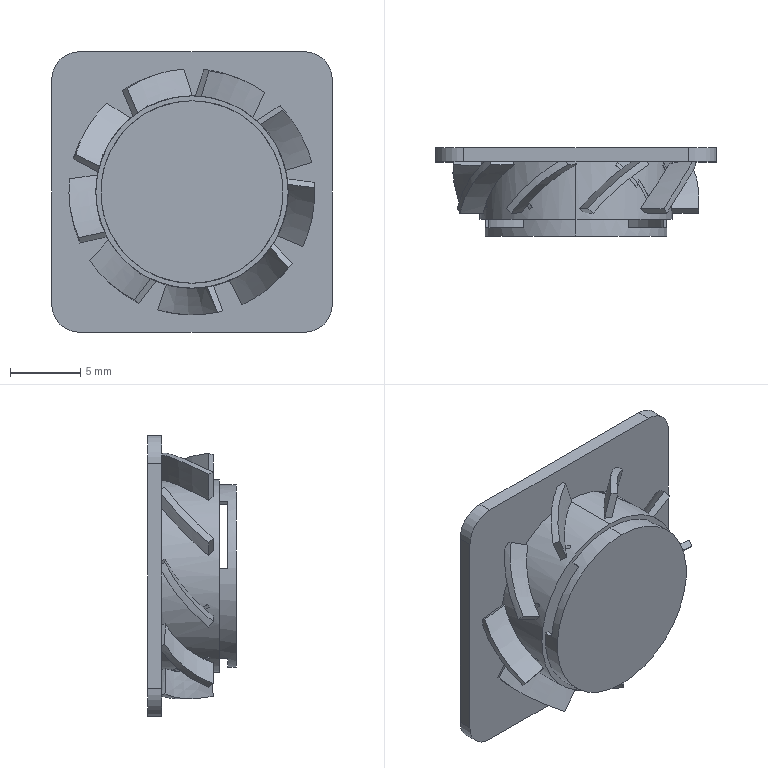Part | SolidWorks | features BaseBody 1, ICE 1 | 1 solid | 133 faces | box 20 x 6.3 x 20 mm | volume 1130 mm3 | spline 105 | plane 15 | cylinder 13 | commonest cylinder face diameters 4 x4 12.5 x4 13.7 x3 13 x2